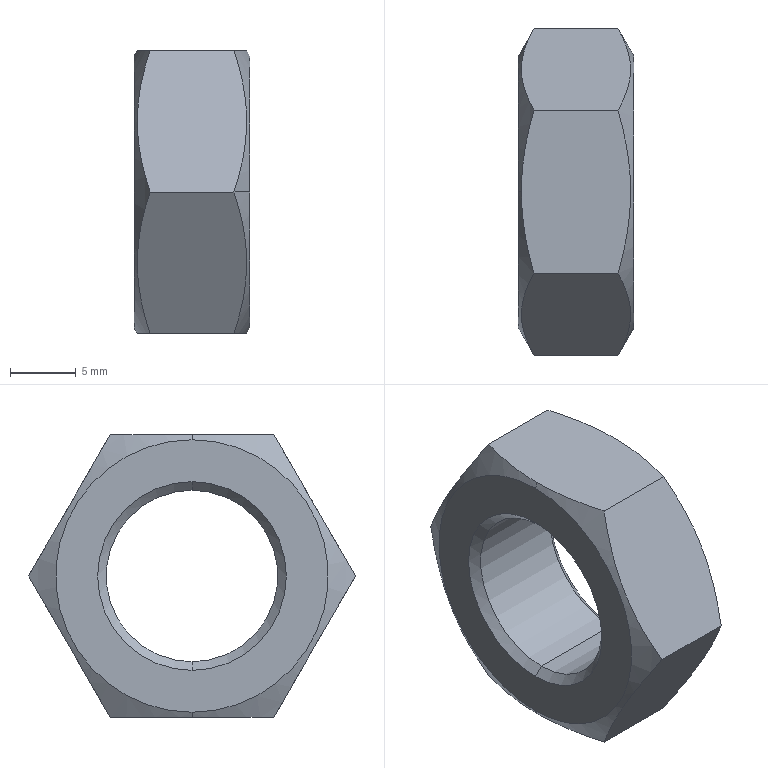Part | SolidWorks | features BaseBody 1 | 1 solid | 18 faces | box 8.8 x 24.942 x 21.6 mm | volume 2306 mm3 | cone 8 | plane 8 | cylinder 2 | commonest cylinder face diameters 13.101 x2
STEP:
#1=CARTESIAN_POINT('',(74.096,407.,46.45));
#2=VERTEX_POINT('',#1);
#3=CARTESIAN_POINT('',(74.096,407.,59.55));
#4=VERTEX_POINT('',#3);
#5=CARTESIAN_POINT('',(74.096,407.,53.));
#6=DIRECTION('',(-1.,0.,0.));
#7=DIRECTION('',(0.,0.,1.));
#8=AXIS2_PLACEMENT_3D('',#5,#6,#7);
#9=CIRCLE('',#8,6.55);
#10=EDGE_CURVE('',#2,#4,#9,.T.);
#11=ORIENTED_EDGE('',*,*,#10,.F.);
#12=CARTESIAN_POINT('',(73.447,407.,45.8));
#13=VERTEX_POINT('',#12);
#14=CARTESIAN_POINT('',(73.447,407.,45.8));
#15=DIRECTION('',(-0.7071,0.,-0.7071));
#16=VECTOR('',#15,1000.);
#17=LINE('',#14,#16);
#18=EDGE_CURVE('',#2,#13,#17,.T.);
#19=ORIENTED_EDGE('',*,*,#18,.T.);
#20=CARTESIAN_POINT('',(73.447,407.,60.2));
#21=VERTEX_POINT('',#20);
#22=CARTESIAN_POINT('',(73.447,407.,53.));
#23=DIRECTION('',(1.,0.,0.));
#24=DIRECTION('',(0.,0.,1.));
#25=AXIS2_PLACEMENT_3D('',#22,#23,#24);
#26=CIRCLE('',#25,7.2);
#27=EDGE_CURVE('',#21,#13,#26,.T.);
#28=ORIENTED_EDGE('',*,*,#27,.F.);
#29=CARTESIAN_POINT('',(73.447,407.,60.2));
#30=DIRECTION('',(-0.7071,0.,0.7071));
#31=VECTOR('',#30,1000.);
#32=LINE('',#29,#31);
#33=EDGE_CURVE('',#4,#21,#32,.T.);
#34=ORIENTED_EDGE('',*,*,#33,.F.);
#35=EDGE_LOOP('',(#11,#19,#28,#34));
#36=FACE_OUTER_BOUND('',#35,.T.);
#37=CARTESIAN_POINT('',(73.447,407.,53.));
#38=DIRECTION('',(-1.,0.,0.));
#39=DIRECTION('',(0.,0.,1.));
#40=AXIS2_PLACEMENT_3D('',#37,#38,#39);
#41=CONICAL_SURFACE('',#40,7.2,0.7854);
#42=ADVANCED_FACE('',(#36),#41,.F.);
#43=CARTESIAN_POINT('',(73.447,407.,63.4));
#44=VERTEX_POINT('',#43);
#45=CARTESIAN_POINT('',(73.447,407.,42.6));
#46=VERTEX_POINT('',#45);
#47=CARTESIAN_POINT('',(73.447,407.,53.));
#48=DIRECTION('',(-1.,0.,0.));
#49=DIRECTION('',(0.,0.,-1.));
#50=AXIS2_PLACEMENT_3D('',#47,#48,#49);
#51=CIRCLE('',#50,10.4);
#52=EDGE_CURVE('',#44,#46,#51,.T.);
#53=ORIENTED_EDGE('',*,*,#52,.F.);
#54=CARTESIAN_POINT('',(73.677,407.,63.8));
#55=VERTEX_POINT('',#54);
#56=CARTESIAN_POINT('',(74.649,407.,65.483));
#57=DIRECTION('',(0.5,0.,0.866));
#58=VECTOR('',#57,1000.);
#59=LINE('',#56,#58);
#60=EDGE_CURVE('',#44,#55,#59,.T.);
#61=ORIENTED_EDGE('',*,*,#60,.T.);
#62=CARTESIAN_POINT('',(74.642,413.235,63.8));
#63=VERTEX_POINT('',#62);
#64=CARTESIAN_POINT('',(73.677,407.,63.8));
#65=CARTESIAN_POINT('',(73.677,408.064,63.8));
#66=CARTESIAN_POINT('',(73.77,409.114,63.8));
#67=CARTESIAN_POINT('',(74.106,411.19,63.8));
#68=CARTESIAN_POINT('',(74.348,412.217,63.8));
#69=CARTESIAN_POINT('',(74.642,413.235,63.8));
#70=B_SPLINE_CURVE_WITH_KNOTS('',3,(#64,#65,#66,#67,#68,#69),.UNSPECIFIED.,.F.,.F.,(4,2,4),(0.00631,0.009464,0.01262),.UNSPECIFIED.);
#71=EDGE_CURVE('',#55,#63,#70,.T.);
#72=ORIENTED_EDGE('',*,*,#71,.T.);
#73=CARTESIAN_POINT('',(74.642,419.471,53.));
#74=VERTEX_POINT('',#73);
#75=CARTESIAN_POINT('',(74.642,413.235,63.8));
#76=CARTESIAN_POINT('',(74.348,413.744,62.918));
#77=CARTESIAN_POINT('',(74.106,414.257,62.03));
#78=CARTESIAN_POINT('',(73.77,415.293,60.235));
#79=CARTESIAN_POINT('',(73.678,415.817,59.329));
#80=CARTESIAN_POINT('',(73.677,416.612,57.951));
#81=CARTESIAN_POINT('',(73.7,416.878,57.49));
#82=CARTESIAN_POINT('',(73.788,417.405,56.578));
#83=CARTESIAN_POINT('',(73.853,417.667,56.124));
#84=CARTESIAN_POINT('',(74.105,418.447,54.773));
#85=CARTESIAN_POINT('',(74.348,418.961,53.883));
#86=CARTESIAN_POINT('',(74.642,419.471,53.));
#87=B_SPLINE_CURVE_WITH_KNOTS('',3,(#75,#76,#77,#78,#79,#80,#81,#82,#83,#84,#85,#86),.UNSPECIFIED.,.F.,.F.,(4,2,2,2,2,4),(0.,0.003149,0.006297,0.007872,0.009446,0.01259),.UNSPECIFIED.);
#88=EDGE_CURVE('',#63,#74,#87,.T.);
#89=ORIENTED_EDGE('',*,*,#88,.T.);
#90=CARTESIAN_POINT('',(74.642,413.235,42.2));
#91=VERTEX_POINT('',#90);
#92=CARTESIAN_POINT('',(74.642,419.471,53.));
#93=CARTESIAN_POINT('',(74.348,418.962,52.118));
#94=CARTESIAN_POINT('',(74.106,418.449,51.23));
#95=CARTESIAN_POINT('',(73.77,417.413,49.435));
#96=CARTESIAN_POINT('',(73.678,416.889,48.529));
#97=CARTESIAN_POINT('',(73.677,416.094,47.151));
#98=CARTESIAN_POINT('',(73.7,415.828,46.69));
#99=CARTESIAN_POINT('',(73.788,415.301,45.778));
#100=CARTESIAN_POINT('',(73.853,415.039,45.324));
#101=CARTESIAN_POINT('',(74.105,414.259,43.973));
#102=CARTESIAN_POINT('',(74.348,413.745,43.083));
#103=CARTESIAN_POINT('',(74.642,413.235,42.2));
#104=B_SPLINE_CURVE_WITH_KNOTS('',3,(#92,#93,#94,#95,#96,#97,#98,#99,#100,#101,#102,#103),.UNSPECIFIED.,.F.,.F.,(4,2,2,2,2,4),(0.,0.003149,0.006297,0.007872,0.009446,0.01259),.UNSPECIFIED.);
#105=EDGE_CURVE('',#74,#91,#104,.T.);
#106=ORIENTED_EDGE('',*,*,#105,.T.);
#107=CARTESIAN_POINT('',(73.677,407.,42.2));
#108=VERTEX_POINT('',#107);
#109=CARTESIAN_POINT('',(74.642,413.235,42.2));
#110=CARTESIAN_POINT('',(74.348,412.217,42.2));
#111=CARTESIAN_POINT('',(74.106,411.19,42.2));
#112=CARTESIAN_POINT('',(73.77,409.114,42.2));
#113=CARTESIAN_POINT('',(73.677,408.064,42.2));
#114=CARTESIAN_POINT('',(73.677,407.,42.2));
#115=B_SPLINE_CURVE_WITH_KNOTS('',3,(#109,#110,#111,#112,#113,#114),.UNSPECIFIED.,.F.,.F.,(4,2,4),(-0.00631,-0.003155,0.),.UNSPECIFIED.);
#116=EDGE_CURVE('',#91,#108,#115,.T.);
#117=ORIENTED_EDGE('',*,*,#116,.T.);
#118=CARTESIAN_POINT('',(74.649,407.,40.517));
#119=DIRECTION('',(0.5,0.,-0.866));
#120=VECTOR('',#119,1000.);
#121=LINE('',#118,#120);
#122=EDGE_CURVE('',#46,#108,#121,.T.);
#123=ORIENTED_EDGE('',*,*,#122,.F.);
#124=EDGE_LOOP('',(#53,#61,#72,#89,#106,#117,#123));
#125=FACE_OUTER_BOUND('',#124,.T.);
#126=CARTESIAN_POINT('',(74.649,407.,53.));
#127=DIRECTION('',(1.,0.,0.));
#128=DIRECTION('',(0.,0.,-1.));
#129=AXIS2_PLACEMENT_3D('',#126,#127,#128);
#130=CONICAL_SURFACE('',#129,12.483,1.047);
#131=ADVANCED_FACE('',(#125),#130,.T.);
#132=CARTESIAN_POINT('',(81.597,407.,46.45));
#133=VERTEX_POINT('',#132);
#134=CARTESIAN_POINT('',(81.597,407.,59.55));
#135=VERTEX_POINT('',#134);
#136=CARTESIAN_POINT('',(81.597,407.,53.));
#137=DIRECTION('',(-1.,0.,0.));
#138=DIRECTION('',(0.,0.,1.));
#139=AXIS2_PLACEMENT_3D('',#136,#137,#138);
#140=CIRCLE('',#139,6.55);
#141=EDGE_CURVE('',#133,#135,#140,.T.);
#142=ORIENTED_EDGE('',*,*,#141,.F.);
#143=CARTESIAN_POINT('',(73.447,407.,46.45));
#144=DIRECTION('',(-1.,0.,0.));
#145=VECTOR('',#144,1000.);
#146=LINE('',#143,#145);
#147=EDGE_CURVE('',#133,#2,#146,.T.);
#148=ORIENTED_EDGE('',*,*,#147,.T.);
#149=ORIENTED_EDGE('',*,*,#10,.T.);
#150=CARTESIAN_POINT('',(73.447,407.,59.55));
#151=DIRECTION('',(-1.,0.,0.));
#152=VECTOR('',#151,1000.);
#153=LINE('',#150,#152);
#154=EDGE_CURVE('',#135,#4,#153,.T.);
#155=ORIENTED_EDGE('',*,*,#154,.F.);
#156=EDGE_LOOP('',(#142,#148,#149,#155));
#157=FACE_OUTER_BOUND('',#156,.T.);
#158=CARTESIAN_POINT('',(73.447,407.,53.));
#159=DIRECTION('',(-1.,0.,0.));
#160=DIRECTION('',(0.,0.,1.));
#161=AXIS2_PLACEMENT_3D('',#158,#159,#160);
#162=CYLINDRICAL_SURFACE('',#161,6.55);
#163=ADVANCED_FACE('',(#157),#162,.F.);
#164=ORIENTED_EDGE('',*,*,#141,.T.);
#165=CARTESIAN_POINT('',(82.247,407.,60.2));
#166=VERTEX_POINT('',#165);
#167=CARTESIAN_POINT('',(82.247,407.,60.2));
#168=DIRECTION('',(0.7071,0.,0.7071));
#169=VECTOR('',#168,1000.);
#170=LINE('',#167,#169);
#171=EDGE_CURVE('',#135,#166,#170,.T.);
#172=ORIENTED_EDGE('',*,*,#171,.T.);
#173=CARTESIAN_POINT('',(82.247,407.,45.8));
#174=VERTEX_POINT('',#173);
#175=CARTESIAN_POINT('',(82.247,407.,53.));
#176=DIRECTION('',(-1.,0.,0.));
#177=DIRECTION('',(0.,0.,-1.));
#178=AXIS2_PLACEMENT_3D('',#175,#176,#177);
#179=CIRCLE('',#178,7.2);
#180=EDGE_CURVE('',#174,#166,#179,.T.);
#181=ORIENTED_EDGE('',*,*,#180,.F.);
#182=CARTESIAN_POINT('',(82.247,407.,45.8));
#183=DIRECTION('',(0.7071,0.,-0.7071));
#184=VECTOR('',#183,1000.);
#185=LINE('',#182,#184);
#186=EDGE_CURVE('',#133,#174,#185,.T.);
#187=ORIENTED_EDGE('',*,*,#186,.F.);
#188=EDGE_LOOP('',(#164,#172,#181,#187));
#189=FACE_OUTER_BOUND('',#188,.T.);
#190=CARTESIAN_POINT('',(82.247,407.,53.));
#191=DIRECTION('',(1.,0.,0.));
#192=DIRECTION('',(0.,0.,-1.));
#193=AXIS2_PLACEMENT_3D('',#190,#191,#192);
#194=CONICAL_SURFACE('',#193,7.2,0.7854);
#195=ADVANCED_FACE('',(#189),#194,.F.);
#196=CARTESIAN_POINT('',(82.247,396.6,53.));
#197=VERTEX_POINT('',#196);
#198=CARTESIAN_POINT('',(82.247,417.4,53.));
#199=VERTEX_POINT('',#198);
#200=CARTESIAN_POINT('',(82.247,407.,53.));
#201=DIRECTION('',(-1.,0.,0.));
#202=DIRECTION('',(0.,-1.,0.));
#203=AXIS2_PLACEMENT_3D('',#200,#201,#202);
#204=CIRCLE('',#203,10.4);
#205=EDGE_CURVE('',#197,#199,#204,.T.);
#206=ORIENTED_EDGE('',*,*,#205,.T.);
#207=CARTESIAN_POINT('',(81.051,419.471,53.));
#208=VERTEX_POINT('',#207);
#209=CARTESIAN_POINT('',(81.044,419.483,53.));
#210=DIRECTION('',(-0.5,0.866,0.));
#211=VECTOR('',#210,1000.);
#212=LINE('',#209,#211);
#213=EDGE_CURVE('',#199,#208,#212,.T.);
#214=ORIENTED_EDGE('',*,*,#213,.T.);
#215=CARTESIAN_POINT('',(81.051,413.235,63.8));
#216=VERTEX_POINT('',#215);
#217=CARTESIAN_POINT('',(81.051,419.471,53.));
#218=CARTESIAN_POINT('',(81.345,418.962,53.882));
#219=CARTESIAN_POINT('',(81.587,418.449,54.77));
#220=CARTESIAN_POINT('',(81.923,417.413,56.565));
#221=CARTESIAN_POINT('',(82.015,416.889,57.471));
#222=CARTESIAN_POINT('',(82.016,416.094,58.849));
#223=CARTESIAN_POINT('',(81.993,415.828,59.31));
#224=CARTESIAN_POINT('',(81.905,415.301,60.222));
#225=CARTESIAN_POINT('',(81.84,415.039,60.676));
#226=CARTESIAN_POINT('',(81.588,414.259,62.027));
#227=CARTESIAN_POINT('',(81.345,413.745,62.917));
#228=CARTESIAN_POINT('',(81.051,413.235,63.8));
#229=B_SPLINE_CURVE_WITH_KNOTS('',3,(#217,#218,#219,#220,#221,#222,#223,#224,#225,#226,#227,#228),.UNSPECIFIED.,.F.,.F.,(4,2,2,2,2,4),(0.,0.003149,0.006297,0.007872,0.009446,0.01259),.UNSPECIFIED.);
#230=EDGE_CURVE('',#208,#216,#229,.T.);
#231=ORIENTED_EDGE('',*,*,#230,.T.);
#232=CARTESIAN_POINT('',(81.051,400.765,63.8));
#233=VERTEX_POINT('',#232);
#234=CARTESIAN_POINT('',(81.051,413.235,63.8));
#235=CARTESIAN_POINT('',(81.345,412.217,63.8));
#236=CARTESIAN_POINT('',(81.588,411.19,63.8));
#237=CARTESIAN_POINT('',(81.923,409.114,63.8));
#238=CARTESIAN_POINT('',(82.016,408.064,63.8));
#239=CARTESIAN_POINT('',(82.016,405.936,63.8));
#240=CARTESIAN_POINT('',(81.923,404.886,63.8));
#241=CARTESIAN_POINT('',(81.588,402.81,63.8));
#242=CARTESIAN_POINT('',(81.345,401.783,63.8));
#243=CARTESIAN_POINT('',(81.051,400.765,63.8));
#244=B_SPLINE_CURVE_WITH_KNOTS('',3,(#234,#235,#236,#237,#238,#239,#240,#241,#242,#243),.UNSPECIFIED.,.F.,.F.,(4,2,2,2,4),(-0.00631,-0.003155,0.,0.003155,0.00631),.UNSPECIFIED.);
#245=EDGE_CURVE('',#216,#233,#244,.T.);
#246=ORIENTED_EDGE('',*,*,#245,.T.);
#247=CARTESIAN_POINT('',(81.051,394.529,53.));
#248=VERTEX_POINT('',#247);
#249=CARTESIAN_POINT('',(81.051,400.765,63.8));
#250=CARTESIAN_POINT('',(81.345,400.256,62.918));
#251=CARTESIAN_POINT('',(81.587,399.743,62.03));
#252=CARTESIAN_POINT('',(81.923,398.707,60.235));
#253=CARTESIAN_POINT('',(82.015,398.183,59.329));
#254=CARTESIAN_POINT('',(82.016,397.388,57.951));
#255=CARTESIAN_POINT('',(81.993,397.122,57.49));
#256=CARTESIAN_POINT('',(81.905,396.595,56.578));
#257=CARTESIAN_POINT('',(81.84,396.333,56.124));
#258=CARTESIAN_POINT('',(81.588,395.553,54.773));
#259=CARTESIAN_POINT('',(81.345,395.039,53.883));
#260=CARTESIAN_POINT('',(81.051,394.529,53.));
#261=B_SPLINE_CURVE_WITH_KNOTS('',3,(#249,#250,#251,#252,#253,#254,#255,#256,#257,#258,#259,#260),.UNSPECIFIED.,.F.,.F.,(4,2,2,2,2,4),(0.,0.003149,0.006297,0.007872,0.009446,0.01259),.UNSPECIFIED.);
#262=EDGE_CURVE('',#233,#248,#261,.T.);
#263=ORIENTED_EDGE('',*,*,#262,.T.);
#264=CARTESIAN_POINT('',(81.044,394.517,53.));
#265=DIRECTION('',(-0.5,-0.866,0.));
#266=VECTOR('',#265,1000.);
#267=LINE('',#264,#266);
#268=EDGE_CURVE('',#197,#248,#267,.T.);
#269=ORIENTED_EDGE('',*,*,#268,.F.);
#270=EDGE_LOOP('',(#206,#214,#231,#246,#263,#269));
#271=FACE_OUTER_BOUND('',#270,.T.);
#272=CARTESIAN_POINT('',(81.044,407.,53.));
#273=DIRECTION('',(-1.,0.,0.));
#274=DIRECTION('',(0.,-1.,0.));
#275=AXIS2_PLACEMENT_3D('',#272,#273,#274);
#276=CONICAL_SURFACE('',#275,12.483,1.047);
#277=ADVANCED_FACE('',(#271),#276,.T.);
#278=ORIENTED_EDGE('',*,*,#27,.T.);
#279=CARTESIAN_POINT('',(73.447,407.,53.));
#280=DIRECTION('',(1.,0.,0.));
#281=DIRECTION('',(0.,0.,1.));
#282=AXIS2_PLACEMENT_3D('',#279,#280,#281);
#283=CIRCLE('',#282,7.2);
#284=EDGE_CURVE('',#13,#21,#283,.T.);
#285=ORIENTED_EDGE('',*,*,#284,.T.);
#286=EDGE_LOOP('',(#278,#285));
#287=FACE_BOUND('',#286,.T.);
#288=CARTESIAN_POINT('',(73.447,407.,53.));
#289=DIRECTION('',(-1.,0.,0.));
#290=DIRECTION('',(0.,0.,-1.));
#291=AXIS2_PLACEMENT_3D('',#288,#289,#290);
#292=CIRCLE('',#291,10.4);
#293=EDGE_CURVE('',#46,#44,#292,.T.);
#294=ORIENTED_EDGE('',*,*,#293,.T.);
#295=ORIENTED_EDGE('',*,*,#52,.T.);
#296=EDGE_LOOP('',(#294,#295));
#297=FACE_OUTER_BOUND('',#296,.T.);
#298=CARTESIAN_POINT('',(73.447,407.,53.));
#299=DIRECTION('',(-1.,0.,0.));
#300=DIRECTION('',(0.,0.,1.));
#301=AXIS2_PLACEMENT_3D('',#298,#299,#300);
#302=PLANE('',#301);
#303=ADVANCED_FACE('',(#287,#297),#302,.T.);
#304=ORIENTED_EDGE('',*,*,#18,.F.);
#305=CARTESIAN_POINT('',(74.096,407.,53.));
#306=DIRECTION('',(-1.,0.,0.));
#307=DIRECTION('',(0.,0.,1.));
#308=AXIS2_PLACEMENT_3D('',#305,#306,#307);
#309=CIRCLE('',#308,6.55);
#310=EDGE_CURVE('',#4,#2,#309,.T.);
#311=ORIENTED_EDGE('',*,*,#310,.F.);
#312=ORIENTED_EDGE('',*,*,#33,.T.);
#313=ORIENTED_EDGE('',*,*,#284,.F.);
#314=EDGE_LOOP('',(#304,#311,#312,#313));
#315=FACE_OUTER_BOUND('',#314,.T.);
#316=CARTESIAN_POINT('',(73.447,407.,53.));
#317=DIRECTION('',(-1.,0.,0.));
#318=DIRECTION('',(0.,0.,1.));
#319=AXIS2_PLACEMENT_3D('',#316,#317,#318);
#320=CONICAL_SURFACE('',#319,7.2,0.7854);
#321=ADVANCED_FACE('',(#315),#320,.F.);
#322=ORIENTED_EDGE('',*,*,#60,.F.);
#323=ORIENTED_EDGE('',*,*,#293,.F.);
#324=ORIENTED_EDGE('',*,*,#122,.T.);
#325=CARTESIAN_POINT('',(74.642,400.765,42.2));
#326=VERTEX_POINT('',#325);
#327=CARTESIAN_POINT('',(73.677,407.,42.2));
#328=CARTESIAN_POINT('',(73.677,405.936,42.2));
#329=CARTESIAN_POINT('',(73.77,404.886,42.2));
#330=CARTESIAN_POINT('',(74.106,402.81,42.2));
#331=CARTESIAN_POINT('',(74.348,401.783,42.2));
#332=CARTESIAN_POINT('',(74.642,400.765,42.2));
#333=B_SPLINE_CURVE_WITH_KNOTS('',3,(#327,#328,#329,#330,#331,#332),.UNSPECIFIED.,.F.,.F.,(4,2,4),(0.,0.003155,0.00631),.UNSPECIFIED.);
#334=EDGE_CURVE('',#108,#326,#333,.T.);
#335=ORIENTED_EDGE('',*,*,#334,.T.);
#336=CARTESIAN_POINT('',(74.642,394.529,53.));
#337=VERTEX_POINT('',#336);
#338=CARTESIAN_POINT('',(74.642,400.765,42.2));
#339=CARTESIAN_POINT('',(74.348,400.256,43.082));
#340=CARTESIAN_POINT('',(74.106,399.743,43.97));
#341=CARTESIAN_POINT('',(73.77,398.707,45.765));
#342=CARTESIAN_POINT('',(73.678,398.183,46.671));
#343=CARTESIAN_POINT('',(73.677,397.388,48.049));
#344=CARTESIAN_POINT('',(73.7,397.122,48.51));
#345=CARTESIAN_POINT('',(73.788,396.595,49.422));
#346=CARTESIAN_POINT('',(73.853,396.333,49.876));
#347=CARTESIAN_POINT('',(74.105,395.553,51.227));
#348=CARTESIAN_POINT('',(74.348,395.039,52.117));
#349=CARTESIAN_POINT('',(74.642,394.529,53.));
#350=B_SPLINE_CURVE_WITH_KNOTS('',3,(#338,#339,#340,#341,#342,#343,#344,#345,#346,#347,#348,#349),.UNSPECIFIED.,.F.,.F.,(4,2,2,2,2,4),(0.,0.003149,0.006297,0.007872,0.009446,0.01259),.UNSPECIFIED.);
#351=EDGE_CURVE('',#326,#337,#350,.T.);
#352=ORIENTED_EDGE('',*,*,#351,.T.);
#353=CARTESIAN_POINT('',(74.642,400.765,63.8));
#354=VERTEX_POINT('',#353);
#355=CARTESIAN_POINT('',(74.642,394.529,53.));
#356=CARTESIAN_POINT('',(74.348,395.038,53.882));
#357=CARTESIAN_POINT('',(74.106,395.551,54.77));
#358=CARTESIAN_POINT('',(73.77,396.587,56.565));
#359=CARTESIAN_POINT('',(73.678,397.111,57.471));
#360=CARTESIAN_POINT('',(73.677,397.906,58.849));
#361=CARTESIAN_POINT('',(73.7,398.172,59.31));
#362=CARTESIAN_POINT('',(73.788,398.699,60.222));
#363=CARTESIAN_POINT('',(73.853,398.961,60.676));
#364=CARTESIAN_POINT('',(74.105,399.741,62.027));
#365=CARTESIAN_POINT('',(74.348,400.255,62.917));
#366=CARTESIAN_POINT('',(74.642,400.765,63.8));
#367=B_SPLINE_CURVE_WITH_KNOTS('',3,(#355,#356,#357,#358,#359,#360,#361,#362,#363,#364,#365,#366),.UNSPECIFIED.,.F.,.F.,(4,2,2,2,2,4),(0.,0.003149,0.006297,0.007872,0.009446,0.01259),.UNSPECIFIED.);
#368=EDGE_CURVE('',#337,#354,#367,.T.);
#369=ORIENTED_EDGE('',*,*,#368,.T.);
#370=CARTESIAN_POINT('',(74.642,400.765,63.8));
#371=CARTESIAN_POINT('',(74.348,401.783,63.8));
#372=CARTESIAN_POINT('',(74.106,402.81,63.8));
#373=CARTESIAN_POINT('',(73.77,404.886,63.8));
#374=CARTESIAN_POINT('',(73.677,405.936,63.8));
#375=CARTESIAN_POINT('',(73.677,407.,63.8));
#376=B_SPLINE_CURVE_WITH_KNOTS('',3,(#370,#371,#372,#373,#374,#375),.UNSPECIFIED.,.F.,.F.,(4,2,4),(0.,0.003155,0.00631),.UNSPECIFIED.);
#377=EDGE_CURVE('',#354,#55,#376,.T.);
#378=ORIENTED_EDGE('',*,*,#377,.T.);
#379=EDGE_LOOP('',(#322,#323,#324,#335,#352,#369,#378));
#380=FACE_OUTER_BOUND('',#379,.T.);
#381=CARTESIAN_POINT('',(74.649,407.,53.));
#382=DIRECTION('',(1.,0.,0.));
#383=DIRECTION('',(0.,0.,-1.));
#384=AXIS2_PLACEMENT_3D('',#381,#382,#383);
#385=CONICAL_SURFACE('',#384,12.483,1.047);
#386=ADVANCED_FACE('',(#380),#385,.T.);
#387=ORIENTED_EDGE('',*,*,#147,.F.);
#388=CARTESIAN_POINT('',(81.597,407.,53.));
#389=DIRECTION('',(-1.,0.,0.));
#390=DIRECTION('',(0.,0.,1.));
#391=AXIS2_PLACEMENT_3D('',#388,#389,#390);
#392=CIRCLE('',#391,6.55);
#393=EDGE_CURVE('',#135,#133,#392,.T.);
#394=ORIENTED_EDGE('',*,*,#393,.F.);
#395=ORIENTED_EDGE('',*,*,#154,.T.);
#396=ORIENTED_EDGE('',*,*,#310,.T.);
#397=EDGE_LOOP('',(#387,#394,#395,#396));
#398=FACE_OUTER_BOUND('',#397,.T.);
#399=CARTESIAN_POINT('',(73.447,407.,53.));
#400=DIRECTION('',(-1.,0.,0.));
#401=DIRECTION('',(0.,0.,1.));
#402=AXIS2_PLACEMENT_3D('',#399,#400,#401);
#403=CYLINDRICAL_SURFACE('',#402,6.55);
#404=ADVANCED_FACE('',(#398),#403,.F.);
#405=ORIENTED_EDGE('',*,*,#245,.F.);
#406=CARTESIAN_POINT('',(73.447,413.235,63.8));
#407=DIRECTION('',(1.,0.,0.));
#408=VECTOR('',#407,1000.);
#409=LINE('',#406,#408);
#410=EDGE_CURVE('',#63,#216,#409,.T.);
#411=ORIENTED_EDGE('',*,*,#410,.F.);
#412=ORIENTED_EDGE('',*,*,#71,.F.);
#413=ORIENTED_EDGE('',*,*,#377,.F.);
#414=CARTESIAN_POINT('',(73.447,400.765,63.8));
#415=DIRECTION('',(-1.,0.,0.));
#416=VECTOR('',#415,1000.);
#417=LINE('',#414,#416);
#418=EDGE_CURVE('',#233,#354,#417,.T.);
#419=ORIENTED_EDGE('',*,*,#418,.F.);
#420=EDGE_LOOP('',(#405,#411,#412,#413,#419));
#421=FACE_OUTER_BOUND('',#420,.T.);
#422=CARTESIAN_POINT('',(73.447,400.765,63.8));
#423=DIRECTION('',(0.,0.,-1.));
#424=DIRECTION('',(-1.,0.,0.));
#425=AXIS2_PLACEMENT_3D('',#422,#423,#424);
#426=PLANE('',#425);
#427=ADVANCED_FACE('',(#421),#426,.F.);
#428=ORIENTED_EDGE('',*,*,#418,.T.);
#429=ORIENTED_EDGE('',*,*,#368,.F.);
#430=CARTESIAN_POINT('',(73.447,394.529,53.));
#431=DIRECTION('',(-1.,0.,0.));
#432=VECTOR('',#431,1000.);
#433=LINE('',#430,#432);
#434=EDGE_CURVE('',#248,#337,#433,.T.);
#435=ORIENTED_EDGE('',*,*,#434,.F.);
#436=ORIENTED_EDGE('',*,*,#262,.F.);
#437=EDGE_LOOP('',(#428,#429,#435,#436));
#438=FACE_OUTER_BOUND('',#437,.T.);
#439=CARTESIAN_POINT('',(73.447,394.529,53.));
#440=DIRECTION('',(0.,0.866,-0.5));
#441=DIRECTION('',(0.,0.5,0.866));
#442=AXIS2_PLACEMENT_3D('',#439,#440,#441);
#443=PLANE('',#442);
#444=ADVANCED_FACE('',(#438),#443,.F.);
#445=ORIENTED_EDGE('',*,*,#434,.T.);
#446=ORIENTED_EDGE('',*,*,#351,.F.);
#447=CARTESIAN_POINT('',(81.051,400.765,42.2));
#448=VERTEX_POINT('',#447);
#449=CARTESIAN_POINT('',(73.447,400.765,42.2));
#450=DIRECTION('',(-1.,0.,0.));
#451=VECTOR('',#450,1000.);
#452=LINE('',#449,#451);
#453=EDGE_CURVE('',#448,#326,#452,.T.);
#454=ORIENTED_EDGE('',*,*,#453,.F.);
#455=CARTESIAN_POINT('',(81.051,394.529,53.));
#456=CARTESIAN_POINT('',(81.345,395.038,52.118));
#457=CARTESIAN_POINT('',(81.587,395.551,51.23));
#458=CARTESIAN_POINT('',(81.923,396.587,49.435));
#459=CARTESIAN_POINT('',(82.015,397.111,48.529));
#460=CARTESIAN_POINT('',(82.016,397.906,47.151));
#461=CARTESIAN_POINT('',(81.993,398.172,46.69));
#462=CARTESIAN_POINT('',(81.905,398.699,45.778));
#463=CARTESIAN_POINT('',(81.84,398.961,45.324));
#464=CARTESIAN_POINT('',(81.588,399.741,43.973));
#465=CARTESIAN_POINT('',(81.345,400.255,43.083));
#466=CARTESIAN_POINT('',(81.051,400.765,42.2));
#467=B_SPLINE_CURVE_WITH_KNOTS('',3,(#455,#456,#457,#458,#459,#460,#461,#462,#463,#464,#465,#466),.UNSPECIFIED.,.F.,.F.,(4,2,2,2,2,4),(0.,0.003149,0.006297,0.007872,0.009446,0.01259),.UNSPECIFIED.);
#468=EDGE_CURVE('',#248,#448,#467,.T.);
#469=ORIENTED_EDGE('',*,*,#468,.F.);
#470=EDGE_LOOP('',(#445,#446,#454,#469));
#471=FACE_OUTER_BOUND('',#470,.T.);
#472=CARTESIAN_POINT('',(73.447,400.765,42.2));
#473=DIRECTION('',(0.,0.866,0.5));
#474=DIRECTION('',(0.,-0.5,0.866));
#475=AXIS2_PLACEMENT_3D('',#472,#473,#474);
#476=PLANE('',#475);
#477=ADVANCED_FACE('',(#471),#476,.F.);
#478=CARTESIAN_POINT('',(81.051,413.235,42.2));
#479=VERTEX_POINT('',#478);
#480=CARTESIAN_POINT('',(81.051,400.765,42.2));
#481=CARTESIAN_POINT('',(81.345,401.783,42.2));
#482=CARTESIAN_POINT('',(81.588,402.81,42.2));
#483=CARTESIAN_POINT('',(81.923,404.886,42.2));
#484=CARTESIAN_POINT('',(82.016,405.936,42.2));
#485=CARTESIAN_POINT('',(82.016,408.064,42.2));
#486=CARTESIAN_POINT('',(81.923,409.114,42.2));
#487=CARTESIAN_POINT('',(81.588,411.19,42.2));
#488=CARTESIAN_POINT('',(81.345,412.217,42.2));
#489=CARTESIAN_POINT('',(81.051,413.235,42.2));
#490=B_SPLINE_CURVE_WITH_KNOTS('',3,(#480,#481,#482,#483,#484,#485,#486,#487,#488,#489),.UNSPECIFIED.,.F.,.F.,(4,2,2,2,4),(-0.00631,-0.003155,0.,0.003155,0.00631),.UNSPECIFIED.);
#491=EDGE_CURVE('',#448,#479,#490,.T.);
#492=ORIENTED_EDGE('',*,*,#491,.F.);
#493=ORIENTED_EDGE('',*,*,#453,.T.);
#494=ORIENTED_EDGE('',*,*,#334,.F.);
#495=ORIENTED_EDGE('',*,*,#116,.F.);
#496=CARTESIAN_POINT('',(73.447,413.235,42.2));
#497=DIRECTION('',(-1.,0.,0.));
#498=VECTOR('',#497,1000.);
#499=LINE('',#496,#498);
#500=EDGE_CURVE('',#479,#91,#499,.T.);
#501=ORIENTED_EDGE('',*,*,#500,.F.);
#502=EDGE_LOOP('',(#492,#493,#494,#495,#501));
#503=FACE_OUTER_BOUND('',#502,.T.);
#504=CARTESIAN_POINT('',(73.447,413.235,42.2));
#505=DIRECTION('',(0.,0.,1.));
#506=DIRECTION('',(1.,0.,0.));
#507=AXIS2_PLACEMENT_3D('',#504,#505,#506);
#508=PLANE('',#507);
#509=ADVANCED_FACE('',(#503),#508,.F.);
#510=ORIENTED_EDGE('',*,*,#500,.T.);
#511=ORIENTED_EDGE('',*,*,#105,.F.);
#512=CARTESIAN_POINT('',(73.447,419.471,53.));
#513=DIRECTION('',(-1.,0.,0.));
#514=VECTOR('',#513,1000.);
#515=LINE('',#512,#514);
#516=EDGE_CURVE('',#208,#74,#515,.T.);
#517=ORIENTED_EDGE('',*,*,#516,.F.);
#518=CARTESIAN_POINT('',(81.051,413.235,42.2));
#519=CARTESIAN_POINT('',(81.345,413.744,43.082));
#520=CARTESIAN_POINT('',(81.587,414.257,43.97));
#521=CARTESIAN_POINT('',(81.923,415.293,45.765));
#522=CARTESIAN_POINT('',(82.015,415.817,46.671));
#523=CARTESIAN_POINT('',(82.016,416.612,48.049));
#524=CARTESIAN_POINT('',(81.993,416.878,48.51));
#525=CARTESIAN_POINT('',(81.905,417.405,49.422));
#526=CARTESIAN_POINT('',(81.84,417.667,49.876));
#527=CARTESIAN_POINT('',(81.588,418.447,51.227));
#528=CARTESIAN_POINT('',(81.345,418.961,52.117));
#529=CARTESIAN_POINT('',(81.051,419.471,53.));
#530=B_SPLINE_CURVE_WITH_KNOTS('',3,(#518,#519,#520,#521,#522,#523,#524,#525,#526,#527,#528,#529),.UNSPECIFIED.,.F.,.F.,(4,2,2,2,2,4),(0.,0.003149,0.006297,0.007872,0.009446,0.01259),.UNSPECIFIED.);
#531=EDGE_CURVE('',#479,#208,#530,.T.);
#532=ORIENTED_EDGE('',*,*,#531,.F.);
#533=EDGE_LOOP('',(#510,#511,#517,#532));
#534=FACE_OUTER_BOUND('',#533,.T.);
#535=CARTESIAN_POINT('',(73.447,419.471,53.));
#536=DIRECTION('',(0.,-0.866,0.5));
#537=DIRECTION('',(0.,-0.5,-0.866));
#538=AXIS2_PLACEMENT_3D('',#535,#536,#537);
#539=PLANE('',#538);
#540=ADVANCED_FACE('',(#534),#539,.F.);
#541=ORIENTED_EDGE('',*,*,#516,.T.);
#542=ORIENTED_EDGE('',*,*,#88,.F.);
#543=ORIENTED_EDGE('',*,*,#410,.T.);
#544=ORIENTED_EDGE('',*,*,#230,.F.);
#545=EDGE_LOOP('',(#541,#542,#543,#544));
#546=FACE_OUTER_BOUND('',#545,.T.);
#547=CARTESIAN_POINT('',(73.447,413.235,63.8));
#548=DIRECTION('',(0.,-0.866,-0.5));
#549=DIRECTION('',(0.,0.5,-0.866));
#550=AXIS2_PLACEMENT_3D('',#547,#548,#549);
#551=PLANE('',#550);
#552=ADVANCED_FACE('',(#546),#551,.F.);
#553=ORIENTED_EDGE('',*,*,#171,.F.);
#554=ORIENTED_EDGE('',*,*,#393,.T.);
#555=ORIENTED_EDGE('',*,*,#186,.T.);
#556=CARTESIAN_POINT('',(82.247,407.,53.));
#557=DIRECTION('',(-1.,0.,0.));
#558=DIRECTION('',(0.,0.,-1.));
#559=AXIS2_PLACEMENT_3D('',#556,#557,#558);
#560=CIRCLE('',#559,7.2);
#561=EDGE_CURVE('',#166,#174,#560,.T.);
#562=ORIENTED_EDGE('',*,*,#561,.F.);
#563=EDGE_LOOP('',(#553,#554,#555,#562));
#564=FACE_OUTER_BOUND('',#563,.T.);
#565=CARTESIAN_POINT('',(82.247,407.,53.));
#566=DIRECTION('',(1.,0.,0.));
#567=DIRECTION('',(0.,0.,-1.));
#568=AXIS2_PLACEMENT_3D('',#565,#566,#567);
#569=CONICAL_SURFACE('',#568,7.2,0.7854);
#570=ADVANCED_FACE('',(#564),#569,.F.);
#571=ORIENTED_EDGE('',*,*,#213,.F.);
#572=CARTESIAN_POINT('',(82.247,407.,53.));
#573=DIRECTION('',(-1.,0.,0.));
#574=DIRECTION('',(0.,-1.,0.));
#575=AXIS2_PLACEMENT_3D('',#572,#573,#574);
#576=CIRCLE('',#575,10.4);
#577=EDGE_CURVE('',#199,#197,#576,.T.);
#578=ORIENTED_EDGE('',*,*,#577,.T.);
#579=ORIENTED_EDGE('',*,*,#268,.T.);
#580=ORIENTED_EDGE('',*,*,#468,.T.);
#581=ORIENTED_EDGE('',*,*,#491,.T.);
#582=ORIENTED_EDGE('',*,*,#531,.T.);
#583=EDGE_LOOP('',(#571,#578,#579,#580,#581,#582));
#584=FACE_OUTER_BOUND('',#583,.T.);
#585=CARTESIAN_POINT('',(81.044,407.,53.));
#586=DIRECTION('',(-1.,0.,0.));
#587=DIRECTION('',(0.,-1.,0.));
#588=AXIS2_PLACEMENT_3D('',#585,#586,#587);
#589=CONICAL_SURFACE('',#588,12.483,1.047);
#590=ADVANCED_FACE('',(#584),#589,.T.);
#591=ORIENTED_EDGE('',*,*,#180,.T.);
#592=ORIENTED_EDGE('',*,*,#561,.T.);
#593=EDGE_LOOP('',(#591,#592));
#594=FACE_BOUND('',#593,.T.);
#595=ORIENTED_EDGE('',*,*,#205,.F.);
#596=ORIENTED_EDGE('',*,*,#577,.F.);
#597=EDGE_LOOP('',(#595,#596));
#598=FACE_OUTER_BOUND('',#597,.T.);
#599=CARTESIAN_POINT('',(82.247,407.,53.));
#600=DIRECTION('',(-1.,0.,0.));
#601=DIRECTION('',(0.,0.,1.));
#602=AXIS2_PLACEMENT_3D('',#599,#600,#601);
#603=PLANE('',#602);
#604=ADVANCED_FACE('',(#594,#598),#603,.F.);
#605=CLOSED_SHELL('',(#42,#131,#163,#195,#277,#303,#321,#386,#404,#427,#444,#477,#509,#540,#552,#570,#590,#604));
#606=MANIFOLD_SOLID_BREP('',#605);
#607=CARTESIAN_POINT('',(0.,0.,0.));
#608=DIRECTION('',(0.,0.,1.));
#609=DIRECTION('',(1.,0.,0.));
#610=AXIS2_PLACEMENT_3D('',#607,#608,#609);
#611=(LENGTH_UNIT()NAMED_UNIT(*)SI_UNIT(.MILLI.,.METRE.));
#612=UNCERTAINTY_MEASURE_WITH_UNIT(LENGTH_MEASURE(0.00001),#611,'','');
#613=(NAMED_UNIT(*)PLANE_ANGLE_UNIT()SI_UNIT($,.RADIAN.));
#614=(NAMED_UNIT(*)SI_UNIT($,.STERADIAN.)SOLID_ANGLE_UNIT());
#615=(GEOMETRIC_REPRESENTATION_CONTEXT(3)GLOBAL_UNCERTAINTY_ASSIGNED_CONTEXT((#612))GLOBAL_UNIT_ASSIGNED_CONTEXT((#611,#613,#614))REPRESENTATION_CONTEXT('',''));
#616=ADVANCED_BREP_SHAPE_REPRESENTATION('',(#606,#610),#615);